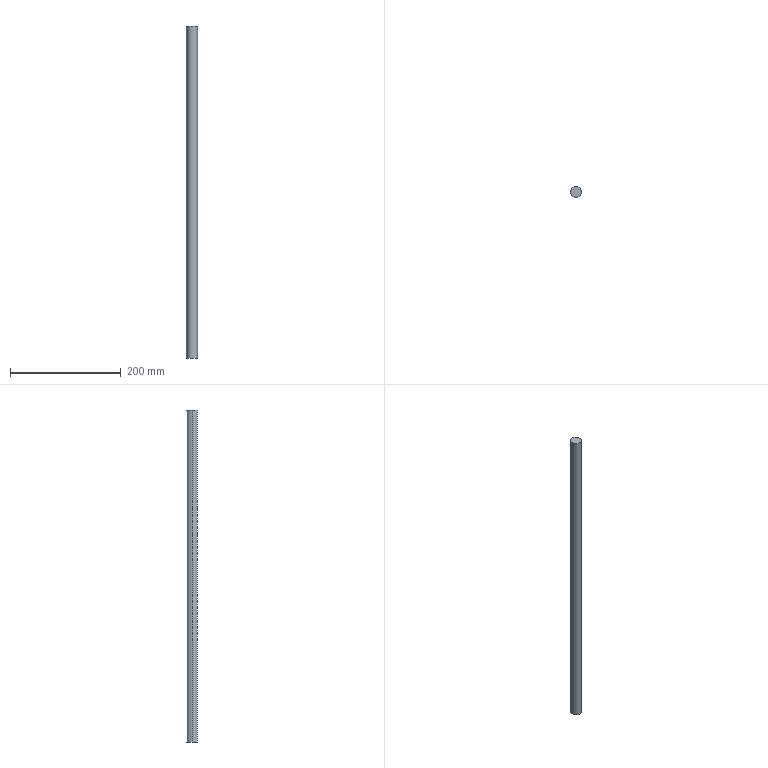Part | SolidWorks | features Extrusion 1 | 1 solid | 4 faces | box 20 x 20 x 600 mm | volume 188496 mm3 | cylinder 2 | plane 2 | commonest cylinder face diameters 20 x2
STEP:
#1=CARTESIAN_POINT('',(10.,0.,300.));
#2=VERTEX_POINT('',#1);
#3=CARTESIAN_POINT('',(-10.,0.,300.));
#4=VERTEX_POINT('',#3);
#5=CARTESIAN_POINT('',(0.,0.,300.));
#6=DIRECTION('',(0.,0.,1.));
#7=DIRECTION('',(1.,0.,0.));
#8=AXIS2_PLACEMENT_3D('',#5,#6,#7);
#9=CIRCLE('',#8,10.);
#10=EDGE_CURVE('',#2,#4,#9,.T.);
#11=ORIENTED_EDGE('',*,*,#10,.F.);
#12=CARTESIAN_POINT('',(10.,0.,-300.));
#13=VERTEX_POINT('',#12);
#14=CARTESIAN_POINT('',(10.,0.,300.));
#15=DIRECTION('',(0.,0.,-1.));
#16=VECTOR('',#15,1000.);
#17=LINE('',#14,#16);
#18=EDGE_CURVE('',#2,#13,#17,.T.);
#19=ORIENTED_EDGE('',*,*,#18,.T.);
#20=CARTESIAN_POINT('',(-10.,0.,-300.));
#21=VERTEX_POINT('',#20);
#22=CARTESIAN_POINT('',(0.,0.,-300.));
#23=DIRECTION('',(0.,0.,1.));
#24=DIRECTION('',(1.,0.,0.));
#25=AXIS2_PLACEMENT_3D('',#22,#23,#24);
#26=CIRCLE('',#25,10.);
#27=EDGE_CURVE('',#13,#21,#26,.T.);
#28=ORIENTED_EDGE('',*,*,#27,.T.);
#29=CARTESIAN_POINT('',(-10.,0.,300.));
#30=DIRECTION('',(0.,0.,-1.));
#31=VECTOR('',#30,1000.);
#32=LINE('',#29,#31);
#33=EDGE_CURVE('',#4,#21,#32,.T.);
#34=ORIENTED_EDGE('',*,*,#33,.F.);
#35=EDGE_LOOP('',(#11,#19,#28,#34));
#36=FACE_OUTER_BOUND('',#35,.T.);
#37=CARTESIAN_POINT('',(0.,0.,300.));
#38=DIRECTION('',(0.,0.,-1.));
#39=DIRECTION('',(-1.,0.,0.));
#40=AXIS2_PLACEMENT_3D('',#37,#38,#39);
#41=CYLINDRICAL_SURFACE('',#40,10.);
#42=ADVANCED_FACE('',(#36),#41,.T.);
#43=ORIENTED_EDGE('',*,*,#18,.F.);
#44=CARTESIAN_POINT('',(0.,0.,300.));
#45=DIRECTION('',(0.,0.,1.));
#46=DIRECTION('',(1.,0.,0.));
#47=AXIS2_PLACEMENT_3D('',#44,#45,#46);
#48=CIRCLE('',#47,10.);
#49=EDGE_CURVE('',#4,#2,#48,.T.);
#50=ORIENTED_EDGE('',*,*,#49,.F.);
#51=ORIENTED_EDGE('',*,*,#33,.T.);
#52=CARTESIAN_POINT('',(0.,0.,-300.));
#53=DIRECTION('',(0.,0.,1.));
#54=DIRECTION('',(1.,0.,0.));
#55=AXIS2_PLACEMENT_3D('',#52,#53,#54);
#56=CIRCLE('',#55,10.);
#57=EDGE_CURVE('',#21,#13,#56,.T.);
#58=ORIENTED_EDGE('',*,*,#57,.T.);
#59=EDGE_LOOP('',(#43,#50,#51,#58));
#60=FACE_OUTER_BOUND('',#59,.T.);
#61=CARTESIAN_POINT('',(0.,0.,300.));
#62=DIRECTION('',(0.,0.,-1.));
#63=DIRECTION('',(-1.,0.,0.));
#64=AXIS2_PLACEMENT_3D('',#61,#62,#63);
#65=CYLINDRICAL_SURFACE('',#64,10.);
#66=ADVANCED_FACE('',(#60),#65,.T.);
#67=ORIENTED_EDGE('',*,*,#49,.T.);
#68=ORIENTED_EDGE('',*,*,#10,.T.);
#69=EDGE_LOOP('',(#67,#68));
#70=FACE_OUTER_BOUND('',#69,.T.);
#71=CARTESIAN_POINT('',(0.,0.,300.));
#72=DIRECTION('',(0.,0.,1.));
#73=DIRECTION('',(1.,0.,0.));
#74=AXIS2_PLACEMENT_3D('',#71,#72,#73);
#75=PLANE('',#74);
#76=ADVANCED_FACE('',(#70),#75,.T.);
#77=ORIENTED_EDGE('',*,*,#57,.F.);
#78=ORIENTED_EDGE('',*,*,#27,.F.);
#79=EDGE_LOOP('',(#77,#78));
#80=FACE_OUTER_BOUND('',#79,.T.);
#81=CARTESIAN_POINT('',(0.,0.,-300.));
#82=DIRECTION('',(0.,0.,1.));
#83=DIRECTION('',(1.,0.,0.));
#84=AXIS2_PLACEMENT_3D('',#81,#82,#83);
#85=PLANE('',#84);
#86=ADVANCED_FACE('',(#80),#85,.F.);
#87=CLOSED_SHELL('',(#42,#66,#76,#86));
#88=MANIFOLD_SOLID_BREP('',#87);
#89=CARTESIAN_POINT('',(0.,0.,0.));
#90=DIRECTION('',(0.,0.,1.));
#91=DIRECTION('',(1.,0.,0.));
#92=AXIS2_PLACEMENT_3D('',#89,#90,#91);
#93=(LENGTH_UNIT()NAMED_UNIT(*)SI_UNIT(.MILLI.,.METRE.));
#94=UNCERTAINTY_MEASURE_WITH_UNIT(LENGTH_MEASURE(0.00001),#93,'','');
#95=(NAMED_UNIT(*)PLANE_ANGLE_UNIT()SI_UNIT($,.RADIAN.));
#96=(NAMED_UNIT(*)SI_UNIT($,.STERADIAN.)SOLID_ANGLE_UNIT());
#97=(GEOMETRIC_REPRESENTATION_CONTEXT(3)GLOBAL_UNCERTAINTY_ASSIGNED_CONTEXT((#94))GLOBAL_UNIT_ASSIGNED_CONTEXT((#93,#95,#96))REPRESENTATION_CONTEXT('',''));
#98=ADVANCED_BREP_SHAPE_REPRESENTATION('',(#88,#92),#97);